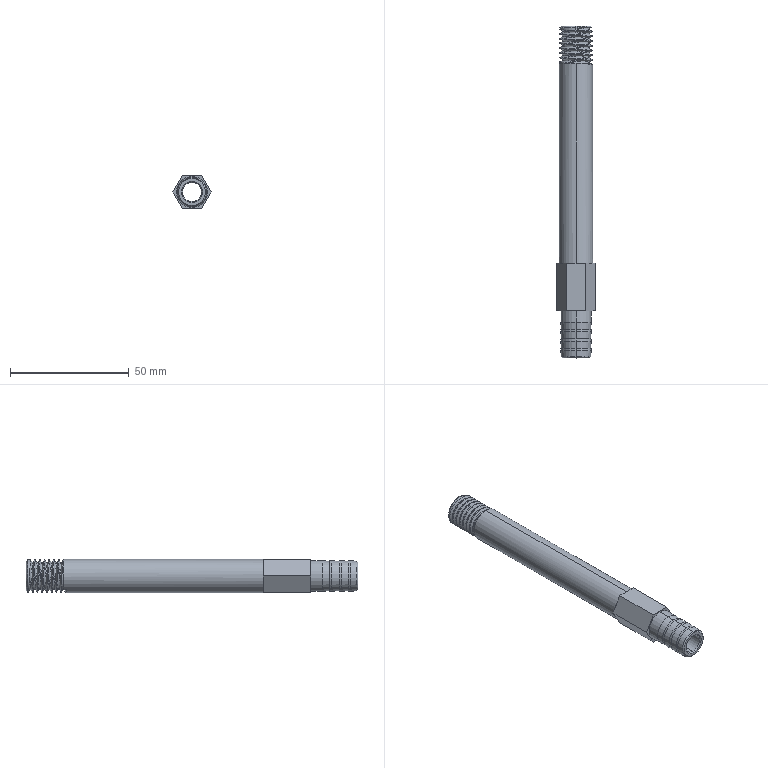Part | SolidWorks | features BaseBody 1 | 1 solid | 82 faces | box 16.166 x 140 x 14 mm | volume 13820 mm3 | cylinder 45 | plane 21 | cone 14 | spline 2 | commonest cylinder face diameters 13.6 x17 11.6 x16 13 x8 8 x2 14 x2